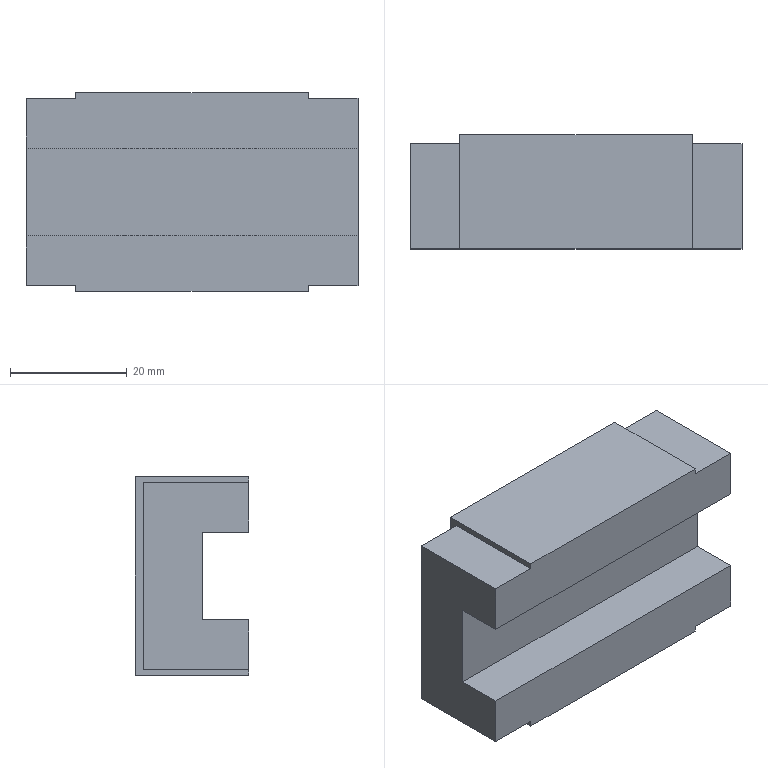Part | NX | 1 solid | 30 faces | box 56.8 x 19.5 x 34 mm | volume 29007 mm3 | plane 18 | cone 8 | cylinder 4 | commonest cylinder face diameters 3.3 x4
STEP:
#1=CARTESIAN_POINT('',(8.5,8.25,-16.));
#2=VERTEX_POINT('',#1);
#3=CARTESIAN_POINT('',(8.5,-9.75,-16.));
#4=VERTEX_POINT('',#3);
#5=CARTESIAN_POINT('',(8.5,8.25,-16.));
#6=DIRECTION('',(0.,-1.,0.));
#7=VECTOR('',#6,1.);
#8=LINE('',#5,#7);
#9=EDGE_CURVE('',#2,#4,#8,.T.);
#10=ORIENTED_EDGE('',*,*,#9,.T.);
#11=CARTESIAN_POINT('',(0.,-9.75,-16.));
#12=VERTEX_POINT('',#11);
#13=CARTESIAN_POINT('',(56.8,-9.75,-16.));
#14=DIRECTION('',(-1.,0.,0.));
#15=VECTOR('',#14,1.);
#16=LINE('',#13,#15);
#17=EDGE_CURVE('',#4,#12,#16,.T.);
#18=ORIENTED_EDGE('',*,*,#17,.T.);
#19=CARTESIAN_POINT('',(0.,8.25,-16.));
#20=VERTEX_POINT('',#19);
#21=CARTESIAN_POINT('',(0.,-9.75,-16.));
#22=DIRECTION('',(0.,1.,0.));
#23=VECTOR('',#22,1.);
#24=LINE('',#21,#23);
#25=EDGE_CURVE('',#12,#20,#24,.T.);
#26=ORIENTED_EDGE('',*,*,#25,.T.);
#27=CARTESIAN_POINT('',(56.8,8.25,-16.));
#28=DIRECTION('',(-1.,0.,0.));
#29=VECTOR('',#28,1.);
#30=LINE('',#27,#29);
#31=EDGE_CURVE('',#2,#20,#30,.T.);
#32=ORIENTED_EDGE('',*,*,#31,.F.);
#33=EDGE_LOOP('',(#10,#18,#26,#32));
#34=FACE_OUTER_BOUND('',#33,.T.);
#35=CARTESIAN_POINT('',(56.8,-9.75,-16.));
#36=DIRECTION('',(0.,0.,1.));
#37=DIRECTION('',(-1.,0.,0.));
#38=AXIS2_PLACEMENT_3D('',#35,#36,#37);
#39=PLANE('',#38);
#40=ADVANCED_FACE('',(#34),#39,.F.);
#41=CARTESIAN_POINT('',(8.5,8.25,16.));
#42=VERTEX_POINT('',#41);
#43=CARTESIAN_POINT('',(8.5,8.25,16.));
#44=DIRECTION('',(0.,0.,-1.));
#45=VECTOR('',#44,1.);
#46=LINE('',#43,#45);
#47=EDGE_CURVE('',#42,#2,#46,.T.);
#48=ORIENTED_EDGE('',*,*,#47,.T.);
#49=ORIENTED_EDGE('',*,*,#31,.T.);
#50=CARTESIAN_POINT('',(0.,8.25,16.));
#51=VERTEX_POINT('',#50);
#52=CARTESIAN_POINT('',(0.,8.25,-16.));
#53=DIRECTION('',(0.,0.,1.));
#54=VECTOR('',#53,1.);
#55=LINE('',#52,#54);
#56=EDGE_CURVE('',#20,#51,#55,.T.);
#57=ORIENTED_EDGE('',*,*,#56,.T.);
#58=CARTESIAN_POINT('',(56.8,8.25,16.));
#59=DIRECTION('',(-1.,0.,0.));
#60=VECTOR('',#59,1.);
#61=LINE('',#58,#60);
#62=EDGE_CURVE('',#42,#51,#61,.T.);
#63=ORIENTED_EDGE('',*,*,#62,.F.);
#64=EDGE_LOOP('',(#48,#49,#57,#63));
#65=FACE_OUTER_BOUND('',#64,.T.);
#66=CARTESIAN_POINT('',(56.8,8.25,-16.));
#67=DIRECTION('',(0.,-1.,0.));
#68=DIRECTION('',(0.,0.,1.));
#69=AXIS2_PLACEMENT_3D('',#66,#67,#68);
#70=PLANE('',#69);
#71=ADVANCED_FACE('',(#65),#70,.F.);
#72=CARTESIAN_POINT('',(8.5,-9.75,16.));
#73=VERTEX_POINT('',#72);
#74=CARTESIAN_POINT('',(8.5,-9.75,16.));
#75=DIRECTION('',(0.,1.,0.));
#76=VECTOR('',#75,1.);
#77=LINE('',#74,#76);
#78=EDGE_CURVE('',#73,#42,#77,.T.);
#79=ORIENTED_EDGE('',*,*,#78,.T.);
#80=ORIENTED_EDGE('',*,*,#62,.T.);
#81=CARTESIAN_POINT('',(0.,-9.75,16.));
#82=VERTEX_POINT('',#81);
#83=CARTESIAN_POINT('',(0.,8.25,16.));
#84=DIRECTION('',(0.,-1.,0.));
#85=VECTOR('',#84,1.);
#86=LINE('',#83,#85);
#87=EDGE_CURVE('',#51,#82,#86,.T.);
#88=ORIENTED_EDGE('',*,*,#87,.T.);
#89=CARTESIAN_POINT('',(56.8,-9.75,16.));
#90=DIRECTION('',(-1.,0.,0.));
#91=VECTOR('',#90,1.);
#92=LINE('',#89,#91);
#93=EDGE_CURVE('',#73,#82,#92,.T.);
#94=ORIENTED_EDGE('',*,*,#93,.F.);
#95=EDGE_LOOP('',(#79,#80,#88,#94));
#96=FACE_OUTER_BOUND('',#95,.T.);
#97=CARTESIAN_POINT('',(56.8,8.25,16.));
#98=DIRECTION('',(0.,0.,-1.));
#99=DIRECTION('',(1.,0.,0.));
#100=AXIS2_PLACEMENT_3D('',#97,#98,#99);
#101=PLANE('',#100);
#102=ADVANCED_FACE('',(#96),#101,.F.);
#103=CARTESIAN_POINT('',(0.,-9.75,-7.5));
#104=VERTEX_POINT('',#103);
#105=CARTESIAN_POINT('',(0.,-9.75,-7.5));
#106=DIRECTION('',(0.,0.,-1.));
#107=VECTOR('',#106,1.);
#108=LINE('',#105,#107);
#109=EDGE_CURVE('',#104,#12,#108,.T.);
#110=ORIENTED_EDGE('',*,*,#109,.T.);
#111=ORIENTED_EDGE('',*,*,#17,.F.);
#112=CARTESIAN_POINT('',(8.5,-9.75,-17.));
#113=VERTEX_POINT('',#112);
#114=CARTESIAN_POINT('',(8.5,-9.75,-16.));
#115=DIRECTION('',(0.,0.,-1.));
#116=VECTOR('',#115,1.);
#117=LINE('',#114,#116);
#118=EDGE_CURVE('',#4,#113,#117,.T.);
#119=ORIENTED_EDGE('',*,*,#118,.T.);
#120=CARTESIAN_POINT('',(48.3,-9.75,-17.));
#121=VERTEX_POINT('',#120);
#122=CARTESIAN_POINT('',(48.3,-9.75,-17.));
#123=DIRECTION('',(-1.,0.,0.));
#124=VECTOR('',#123,1.);
#125=LINE('',#122,#124);
#126=EDGE_CURVE('',#121,#113,#125,.T.);
#127=ORIENTED_EDGE('',*,*,#126,.F.);
#128=CARTESIAN_POINT('',(48.3,-9.75,-16.));
#129=VERTEX_POINT('',#128);
#130=CARTESIAN_POINT('',(48.3,-9.75,-16.));
#131=DIRECTION('',(0.,0.,-1.));
#132=VECTOR('',#131,1.);
#133=LINE('',#130,#132);
#134=EDGE_CURVE('',#129,#121,#133,.T.);
#135=ORIENTED_EDGE('',*,*,#134,.F.);
#136=CARTESIAN_POINT('',(56.8,-9.75,-16.));
#137=VERTEX_POINT('',#136);
#138=CARTESIAN_POINT('',(56.8,-9.75,-16.));
#139=DIRECTION('',(-1.,0.,0.));
#140=VECTOR('',#139,1.);
#141=LINE('',#138,#140);
#142=EDGE_CURVE('',#137,#129,#141,.T.);
#143=ORIENTED_EDGE('',*,*,#142,.F.);
#144=CARTESIAN_POINT('',(56.8,-9.75,-7.5));
#145=VERTEX_POINT('',#144);
#146=CARTESIAN_POINT('',(56.8,-9.75,-7.5));
#147=DIRECTION('',(0.,0.,-1.));
#148=VECTOR('',#147,1.);
#149=LINE('',#146,#148);
#150=EDGE_CURVE('',#145,#137,#149,.T.);
#151=ORIENTED_EDGE('',*,*,#150,.F.);
#152=CARTESIAN_POINT('',(56.8,-9.75,-7.5));
#153=DIRECTION('',(-1.,0.,0.));
#154=VECTOR('',#153,1.);
#155=LINE('',#152,#154);
#156=EDGE_CURVE('',#145,#104,#155,.T.);
#157=ORIENTED_EDGE('',*,*,#156,.T.);
#158=EDGE_LOOP('',(#110,#111,#119,#127,#135,#143,#151,#157));
#159=FACE_OUTER_BOUND('',#158,.T.);
#160=CARTESIAN_POINT('',(56.8,-9.75,-7.5));
#161=DIRECTION('',(0.,1.,0.));
#162=DIRECTION('',(0.,0.,-1.));
#163=AXIS2_PLACEMENT_3D('',#160,#161,#162);
#164=PLANE('',#163);
#165=ADVANCED_FACE('',(#159),#164,.F.);
#166=ORIENTED_EDGE('',*,*,#142,.T.);
#167=CARTESIAN_POINT('',(48.3,8.25,-16.));
#168=VERTEX_POINT('',#167);
#169=CARTESIAN_POINT('',(48.3,8.25,-16.));
#170=DIRECTION('',(0.,-1.,0.));
#171=VECTOR('',#170,1.);
#172=LINE('',#169,#171);
#173=EDGE_CURVE('',#168,#129,#172,.T.);
#174=ORIENTED_EDGE('',*,*,#173,.F.);
#175=CARTESIAN_POINT('',(56.8,8.25,-16.));
#176=VERTEX_POINT('',#175);
#177=CARTESIAN_POINT('',(56.8,8.25,-16.));
#178=DIRECTION('',(-1.,0.,0.));
#179=VECTOR('',#178,1.);
#180=LINE('',#177,#179);
#181=EDGE_CURVE('',#176,#168,#180,.T.);
#182=ORIENTED_EDGE('',*,*,#181,.F.);
#183=CARTESIAN_POINT('',(56.8,-9.75,-16.));
#184=DIRECTION('',(0.,1.,0.));
#185=VECTOR('',#184,1.);
#186=LINE('',#183,#185);
#187=EDGE_CURVE('',#137,#176,#186,.T.);
#188=ORIENTED_EDGE('',*,*,#187,.F.);
#189=EDGE_LOOP('',(#166,#174,#182,#188));
#190=FACE_OUTER_BOUND('',#189,.T.);
#191=CARTESIAN_POINT('',(56.8,-9.75,-16.));
#192=DIRECTION('',(0.,0.,1.));
#193=DIRECTION('',(-1.,0.,0.));
#194=AXIS2_PLACEMENT_3D('',#191,#192,#193);
#195=PLANE('',#194);
#196=ADVANCED_FACE('',(#190),#195,.F.);
#197=ORIENTED_EDGE('',*,*,#181,.T.);
#198=CARTESIAN_POINT('',(48.3,8.25,16.));
#199=VERTEX_POINT('',#198);
#200=CARTESIAN_POINT('',(48.3,8.25,16.));
#201=DIRECTION('',(0.,0.,-1.));
#202=VECTOR('',#201,1.);
#203=LINE('',#200,#202);
#204=EDGE_CURVE('',#199,#168,#203,.T.);
#205=ORIENTED_EDGE('',*,*,#204,.F.);
#206=CARTESIAN_POINT('',(56.8,8.25,16.));
#207=VERTEX_POINT('',#206);
#208=CARTESIAN_POINT('',(56.8,8.25,16.));
#209=DIRECTION('',(-1.,0.,0.));
#210=VECTOR('',#209,1.);
#211=LINE('',#208,#210);
#212=EDGE_CURVE('',#207,#199,#211,.T.);
#213=ORIENTED_EDGE('',*,*,#212,.F.);
#214=CARTESIAN_POINT('',(56.8,8.25,-16.));
#215=DIRECTION('',(0.,0.,1.));
#216=VECTOR('',#215,1.);
#217=LINE('',#214,#216);
#218=EDGE_CURVE('',#176,#207,#217,.T.);
#219=ORIENTED_EDGE('',*,*,#218,.F.);
#220=EDGE_LOOP('',(#197,#205,#213,#219));
#221=FACE_OUTER_BOUND('',#220,.T.);
#222=CARTESIAN_POINT('',(56.8,8.25,-16.));
#223=DIRECTION('',(0.,-1.,0.));
#224=DIRECTION('',(0.,0.,1.));
#225=AXIS2_PLACEMENT_3D('',#222,#223,#224);
#226=PLANE('',#225);
#227=ADVANCED_FACE('',(#221),#226,.F.);
#228=ORIENTED_EDGE('',*,*,#212,.T.);
#229=CARTESIAN_POINT('',(48.3,-9.75,16.));
#230=VERTEX_POINT('',#229);
#231=CARTESIAN_POINT('',(48.3,-9.75,16.));
#232=DIRECTION('',(0.,1.,0.));
#233=VECTOR('',#232,1.);
#234=LINE('',#231,#233);
#235=EDGE_CURVE('',#230,#199,#234,.T.);
#236=ORIENTED_EDGE('',*,*,#235,.F.);
#237=CARTESIAN_POINT('',(56.8,-9.75,16.));
#238=VERTEX_POINT('',#237);
#239=CARTESIAN_POINT('',(56.8,-9.75,16.));
#240=DIRECTION('',(-1.,0.,0.));
#241=VECTOR('',#240,1.);
#242=LINE('',#239,#241);
#243=EDGE_CURVE('',#238,#230,#242,.T.);
#244=ORIENTED_EDGE('',*,*,#243,.F.);
#245=CARTESIAN_POINT('',(56.8,8.25,16.));
#246=DIRECTION('',(0.,-1.,0.));
#247=VECTOR('',#246,1.);
#248=LINE('',#245,#247);
#249=EDGE_CURVE('',#207,#238,#248,.T.);
#250=ORIENTED_EDGE('',*,*,#249,.F.);
#251=EDGE_LOOP('',(#228,#236,#244,#250));
#252=FACE_OUTER_BOUND('',#251,.T.);
#253=CARTESIAN_POINT('',(56.8,8.25,16.));
#254=DIRECTION('',(0.,0.,-1.));
#255=DIRECTION('',(1.,0.,0.));
#256=AXIS2_PLACEMENT_3D('',#253,#254,#255);
#257=PLANE('',#256);
#258=ADVANCED_FACE('',(#252),#257,.F.);
#259=CARTESIAN_POINT('',(0.,-9.75,7.5));
#260=VERTEX_POINT('',#259);
#261=CARTESIAN_POINT('',(0.,-9.75,16.));
#262=DIRECTION('',(0.,0.,-1.));
#263=VECTOR('',#262,1.);
#264=LINE('',#261,#263);
#265=EDGE_CURVE('',#82,#260,#264,.T.);
#266=ORIENTED_EDGE('',*,*,#265,.T.);
#267=CARTESIAN_POINT('',(56.8,-9.75,7.5));
#268=VERTEX_POINT('',#267);
#269=CARTESIAN_POINT('',(56.8,-9.75,7.5));
#270=DIRECTION('',(-1.,0.,0.));
#271=VECTOR('',#270,1.);
#272=LINE('',#269,#271);
#273=EDGE_CURVE('',#268,#260,#272,.T.);
#274=ORIENTED_EDGE('',*,*,#273,.F.);
#275=CARTESIAN_POINT('',(56.8,-9.75,16.));
#276=DIRECTION('',(0.,0.,-1.));
#277=VECTOR('',#276,1.);
#278=LINE('',#275,#277);
#279=EDGE_CURVE('',#238,#268,#278,.T.);
#280=ORIENTED_EDGE('',*,*,#279,.F.);
#281=ORIENTED_EDGE('',*,*,#243,.T.);
#282=CARTESIAN_POINT('',(48.3,-9.75,17.));
#283=VERTEX_POINT('',#282);
#284=CARTESIAN_POINT('',(48.3,-9.75,17.));
#285=DIRECTION('',(0.,0.,-1.));
#286=VECTOR('',#285,1.);
#287=LINE('',#284,#286);
#288=EDGE_CURVE('',#283,#230,#287,.T.);
#289=ORIENTED_EDGE('',*,*,#288,.F.);
#290=CARTESIAN_POINT('',(8.5,-9.75,17.));
#291=VERTEX_POINT('',#290);
#292=CARTESIAN_POINT('',(48.3,-9.75,17.));
#293=DIRECTION('',(-1.,0.,0.));
#294=VECTOR('',#293,1.);
#295=LINE('',#292,#294);
#296=EDGE_CURVE('',#283,#291,#295,.T.);
#297=ORIENTED_EDGE('',*,*,#296,.T.);
#298=CARTESIAN_POINT('',(8.5,-9.75,17.));
#299=DIRECTION('',(0.,0.,-1.));
#300=VECTOR('',#299,1.);
#301=LINE('',#298,#300);
#302=EDGE_CURVE('',#291,#73,#301,.T.);
#303=ORIENTED_EDGE('',*,*,#302,.T.);
#304=ORIENTED_EDGE('',*,*,#93,.T.);
#305=EDGE_LOOP('',(#266,#274,#280,#281,#289,#297,#303,#304));
#306=FACE_OUTER_BOUND('',#305,.T.);
#307=CARTESIAN_POINT('',(56.8,-9.75,16.));
#308=DIRECTION('',(0.,1.,0.));
#309=DIRECTION('',(0.,0.,-1.));
#310=AXIS2_PLACEMENT_3D('',#307,#308,#309);
#311=PLANE('',#310);
#312=ADVANCED_FACE('',(#306),#311,.F.);
#313=CARTESIAN_POINT('',(0.,-1.75,7.5));
#314=VERTEX_POINT('',#313);
#315=CARTESIAN_POINT('',(0.,-9.75,7.5));
#316=DIRECTION('',(0.,1.,0.));
#317=VECTOR('',#316,1.);
#318=LINE('',#315,#317);
#319=EDGE_CURVE('',#260,#314,#318,.T.);
#320=ORIENTED_EDGE('',*,*,#319,.T.);
#321=CARTESIAN_POINT('',(56.8,-1.75,7.5));
#322=VERTEX_POINT('',#321);
#323=CARTESIAN_POINT('',(56.8,-1.75,7.5));
#324=DIRECTION('',(-1.,0.,0.));
#325=VECTOR('',#324,1.);
#326=LINE('',#323,#325);
#327=EDGE_CURVE('',#322,#314,#326,.T.);
#328=ORIENTED_EDGE('',*,*,#327,.F.);
#329=CARTESIAN_POINT('',(56.8,-9.75,7.5));
#330=DIRECTION('',(0.,1.,0.));
#331=VECTOR('',#330,1.);
#332=LINE('',#329,#331);
#333=EDGE_CURVE('',#268,#322,#332,.T.);
#334=ORIENTED_EDGE('',*,*,#333,.F.);
#335=ORIENTED_EDGE('',*,*,#273,.T.);
#336=EDGE_LOOP('',(#320,#328,#334,#335));
#337=FACE_OUTER_BOUND('',#336,.T.);
#338=CARTESIAN_POINT('',(56.8,-9.75,7.5));
#339=DIRECTION('',(0.,0.,1.));
#340=DIRECTION('',(0.,1.,0.));
#341=AXIS2_PLACEMENT_3D('',#338,#339,#340);
#342=PLANE('',#341);
#343=ADVANCED_FACE('',(#337),#342,.F.);
#344=CARTESIAN_POINT('',(0.,-1.75,-7.5));
#345=VERTEX_POINT('',#344);
#346=CARTESIAN_POINT('',(0.,-1.75,7.5));
#347=DIRECTION('',(0.,0.,-1.));
#348=VECTOR('',#347,1.);
#349=LINE('',#346,#348);
#350=EDGE_CURVE('',#314,#345,#349,.T.);
#351=ORIENTED_EDGE('',*,*,#350,.T.);
#352=CARTESIAN_POINT('',(56.8,-1.75,-7.5));
#353=VERTEX_POINT('',#352);
#354=CARTESIAN_POINT('',(56.8,-1.75,-7.5));
#355=DIRECTION('',(-1.,0.,0.));
#356=VECTOR('',#355,1.);
#357=LINE('',#354,#356);
#358=EDGE_CURVE('',#353,#345,#357,.T.);
#359=ORIENTED_EDGE('',*,*,#358,.F.);
#360=CARTESIAN_POINT('',(56.8,-1.75,7.5));
#361=DIRECTION('',(0.,0.,-1.));
#362=VECTOR('',#361,1.);
#363=LINE('',#360,#362);
#364=EDGE_CURVE('',#322,#353,#363,.T.);
#365=ORIENTED_EDGE('',*,*,#364,.F.);
#366=ORIENTED_EDGE('',*,*,#327,.T.);
#367=EDGE_LOOP('',(#351,#359,#365,#366));
#368=FACE_OUTER_BOUND('',#367,.T.);
#369=CARTESIAN_POINT('',(56.8,-1.75,7.5));
#370=DIRECTION('',(0.,1.,0.));
#371=DIRECTION('',(0.,0.,-1.));
#372=AXIS2_PLACEMENT_3D('',#369,#370,#371);
#373=PLANE('',#372);
#374=ADVANCED_FACE('',(#368),#373,.F.);
#375=CARTESIAN_POINT('',(0.,-1.75,-7.5));
#376=DIRECTION('',(0.,-1.,0.));
#377=VECTOR('',#376,1.);
#378=LINE('',#375,#377);
#379=EDGE_CURVE('',#345,#104,#378,.T.);
#380=ORIENTED_EDGE('',*,*,#379,.T.);
#381=ORIENTED_EDGE('',*,*,#156,.F.);
#382=CARTESIAN_POINT('',(56.8,-1.75,-7.5));
#383=DIRECTION('',(0.,-1.,0.));
#384=VECTOR('',#383,1.);
#385=LINE('',#382,#384);
#386=EDGE_CURVE('',#353,#145,#385,.T.);
#387=ORIENTED_EDGE('',*,*,#386,.F.);
#388=ORIENTED_EDGE('',*,*,#358,.T.);
#389=EDGE_LOOP('',(#380,#381,#387,#388));
#390=FACE_OUTER_BOUND('',#389,.T.);
#391=CARTESIAN_POINT('',(56.8,-1.75,-7.5));
#392=DIRECTION('',(0.,0.,-1.));
#393=DIRECTION('',(0.,-1.,0.));
#394=AXIS2_PLACEMENT_3D('',#391,#392,#393);
#395=PLANE('',#394);
#396=ADVANCED_FACE('',(#390),#395,.F.);
#397=ORIENTED_EDGE('',*,*,#150,.T.);
#398=ORIENTED_EDGE('',*,*,#187,.T.);
#399=ORIENTED_EDGE('',*,*,#218,.T.);
#400=ORIENTED_EDGE('',*,*,#249,.T.);
#401=ORIENTED_EDGE('',*,*,#279,.T.);
#402=ORIENTED_EDGE('',*,*,#333,.T.);
#403=ORIENTED_EDGE('',*,*,#364,.T.);
#404=ORIENTED_EDGE('',*,*,#386,.T.);
#405=EDGE_LOOP('',(#397,#398,#399,#400,#401,#402,#403,#404));
#406=FACE_OUTER_BOUND('',#405,.T.);
#407=CARTESIAN_POINT('',(56.8,0.,0.));
#408=DIRECTION('',(1.,0.,0.));
#409=DIRECTION('',(0.,0.,1.));
#410=AXIS2_PLACEMENT_3D('',#407,#408,#409);
#411=PLANE('',#410);
#412=ADVANCED_FACE('',(#406),#411,.T.);
#413=ORIENTED_EDGE('',*,*,#109,.F.);
#414=ORIENTED_EDGE('',*,*,#379,.F.);
#415=ORIENTED_EDGE('',*,*,#350,.F.);
#416=ORIENTED_EDGE('',*,*,#319,.F.);
#417=ORIENTED_EDGE('',*,*,#265,.F.);
#418=ORIENTED_EDGE('',*,*,#87,.F.);
#419=ORIENTED_EDGE('',*,*,#56,.F.);
#420=ORIENTED_EDGE('',*,*,#25,.F.);
#421=EDGE_LOOP('',(#413,#414,#415,#416,#417,#418,#419,#420));
#422=FACE_OUTER_BOUND('',#421,.T.);
#423=CARTESIAN_POINT('',(0.,0.,0.));
#424=DIRECTION('',(1.,0.,0.));
#425=DIRECTION('',(0.,0.,1.));
#426=AXIS2_PLACEMENT_3D('',#423,#424,#425);
#427=PLANE('',#426);
#428=ADVANCED_FACE('',(#422),#427,.F.);
#429=CARTESIAN_POINT('',(8.5,9.75,-17.));
#430=VERTEX_POINT('',#429);
#431=CARTESIAN_POINT('',(8.5,-9.75,-17.));
#432=DIRECTION('',(0.,1.,0.));
#433=VECTOR('',#432,1.);
#434=LINE('',#431,#433);
#435=EDGE_CURVE('',#113,#430,#434,.T.);
#436=ORIENTED_EDGE('',*,*,#435,.T.);
#437=CARTESIAN_POINT('',(48.3,9.75,-17.));
#438=VERTEX_POINT('',#437);
#439=CARTESIAN_POINT('',(48.3,9.75,-17.));
#440=DIRECTION('',(-1.,0.,0.));
#441=VECTOR('',#440,1.);
#442=LINE('',#439,#441);
#443=EDGE_CURVE('',#438,#430,#442,.T.);
#444=ORIENTED_EDGE('',*,*,#443,.F.);
#445=CARTESIAN_POINT('',(48.3,-9.75,-17.));
#446=DIRECTION('',(0.,1.,0.));
#447=VECTOR('',#446,1.);
#448=LINE('',#445,#447);
#449=EDGE_CURVE('',#121,#438,#448,.T.);
#450=ORIENTED_EDGE('',*,*,#449,.F.);
#451=ORIENTED_EDGE('',*,*,#126,.T.);
#452=EDGE_LOOP('',(#436,#444,#450,#451));
#453=FACE_OUTER_BOUND('',#452,.T.);
#454=CARTESIAN_POINT('',(48.3,-9.75,-17.));
#455=DIRECTION('',(0.,0.,1.));
#456=DIRECTION('',(-1.,0.,0.));
#457=AXIS2_PLACEMENT_3D('',#454,#455,#456);
#458=PLANE('',#457);
#459=ADVANCED_FACE('',(#453),#458,.F.);
#460=CARTESIAN_POINT('',(41.4,9.75,11.));
#461=VERTEX_POINT('',#460);
#462=CARTESIAN_POINT('',(41.4,9.75,13.));
#463=DIRECTION('',(0.,-1.,0.));
#464=DIRECTION('',(0.,0.,-1.));
#465=AXIS2_PLACEMENT_3D('',#462,#463,#464);
#466=CIRCLE('',#465,2.);
#467=EDGE_CURVE('',#461,#461,#466,.T.);
#468=ORIENTED_EDGE('',*,*,#467,.T.);
#469=EDGE_LOOP('',(#468));
#470=FACE_BOUND('',#469,.T.);
#471=CARTESIAN_POINT('',(41.4,9.75,-15.));
#472=VERTEX_POINT('',#471);
#473=CARTESIAN_POINT('',(41.4,9.75,-13.));
#474=DIRECTION('',(0.,-1.,0.));
#475=DIRECTION('',(0.,0.,-1.));
#476=AXIS2_PLACEMENT_3D('',#473,#474,#475);
#477=CIRCLE('',#476,2.);
#478=EDGE_CURVE('',#472,#472,#477,.T.);
#479=ORIENTED_EDGE('',*,*,#478,.T.);
#480=EDGE_LOOP('',(#479));
#481=FACE_BOUND('',#480,.T.);
#482=CARTESIAN_POINT('',(15.4,9.75,11.));
#483=VERTEX_POINT('',#482);
#484=CARTESIAN_POINT('',(15.4,9.75,13.));
#485=DIRECTION('',(0.,-1.,0.));
#486=DIRECTION('',(0.,0.,-1.));
#487=AXIS2_PLACEMENT_3D('',#484,#485,#486);
#488=CIRCLE('',#487,2.);
#489=EDGE_CURVE('',#483,#483,#488,.T.);
#490=ORIENTED_EDGE('',*,*,#489,.T.);
#491=EDGE_LOOP('',(#490));
#492=FACE_BOUND('',#491,.T.);
#493=CARTESIAN_POINT('',(15.4,9.75,-15.));
#494=VERTEX_POINT('',#493);
#495=CARTESIAN_POINT('',(15.4,9.75,-13.));
#496=DIRECTION('',(0.,-1.,0.));
#497=DIRECTION('',(0.,0.,-1.));
#498=AXIS2_PLACEMENT_3D('',#495,#496,#497);
#499=CIRCLE('',#498,2.);
#500=EDGE_CURVE('',#494,#494,#499,.T.);
#501=ORIENTED_EDGE('',*,*,#500,.T.);
#502=EDGE_LOOP('',(#501));
#503=FACE_BOUND('',#502,.T.);
#504=CARTESIAN_POINT('',(8.5,9.75,17.));
#505=VERTEX_POINT('',#504);
#506=CARTESIAN_POINT('',(8.5,9.75,-17.));
#507=DIRECTION('',(0.,0.,1.));
#508=VECTOR('',#507,1.);
#509=LINE('',#506,#508);
#510=EDGE_CURVE('',#430,#505,#509,.T.);
#511=ORIENTED_EDGE('',*,*,#510,.T.);
#512=CARTESIAN_POINT('',(48.3,9.75,17.));
#513=VERTEX_POINT('',#512);
#514=CARTESIAN_POINT('',(48.3,9.75,17.));
#515=DIRECTION('',(-1.,0.,0.));
#516=VECTOR('',#515,1.);
#517=LINE('',#514,#516);
#518=EDGE_CURVE('',#513,#505,#517,.T.);
#519=ORIENTED_EDGE('',*,*,#518,.F.);
#520=CARTESIAN_POINT('',(48.3,9.75,-17.));
#521=DIRECTION('',(0.,0.,1.));
#522=VECTOR('',#521,1.);
#523=LINE('',#520,#522);
#524=EDGE_CURVE('',#438,#513,#523,.T.);
#525=ORIENTED_EDGE('',*,*,#524,.F.);
#526=ORIENTED_EDGE('',*,*,#443,.T.);
#527=EDGE_LOOP('',(#511,#519,#525,#526));
#528=FACE_BOUND('',#527,.T.);
#529=CARTESIAN_POINT('',(48.3,9.75,-17.));
#530=DIRECTION('',(0.,-1.,0.));
#531=DIRECTION('',(0.,0.,1.));
#532=AXIS2_PLACEMENT_3D('',#529,#530,#531);
#533=PLANE('',#532);
#534=ADVANCED_FACE('',(#470,#481,#492,#503,#528),#533,.F.);
#535=CARTESIAN_POINT('',(8.5,9.75,17.));
#536=DIRECTION('',(0.,-1.,0.));
#537=VECTOR('',#536,1.);
#538=LINE('',#535,#537);
#539=EDGE_CURVE('',#505,#291,#538,.T.);
#540=ORIENTED_EDGE('',*,*,#539,.T.);
#541=ORIENTED_EDGE('',*,*,#296,.F.);
#542=CARTESIAN_POINT('',(48.3,9.75,17.));
#543=DIRECTION('',(0.,-1.,0.));
#544=VECTOR('',#543,1.);
#545=LINE('',#542,#544);
#546=EDGE_CURVE('',#513,#283,#545,.T.);
#547=ORIENTED_EDGE('',*,*,#546,.F.);
#548=ORIENTED_EDGE('',*,*,#518,.T.);
#549=EDGE_LOOP('',(#540,#541,#547,#548));
#550=FACE_OUTER_BOUND('',#549,.T.);
#551=CARTESIAN_POINT('',(48.3,9.75,17.));
#552=DIRECTION('',(0.,0.,-1.));
#553=DIRECTION('',(1.,0.,0.));
#554=AXIS2_PLACEMENT_3D('',#551,#552,#553);
#555=PLANE('',#554);
#556=ADVANCED_FACE('',(#550),#555,.F.);
#557=ORIENTED_EDGE('',*,*,#134,.T.);
#558=ORIENTED_EDGE('',*,*,#449,.T.);
#559=ORIENTED_EDGE('',*,*,#524,.T.);
#560=ORIENTED_EDGE('',*,*,#546,.T.);
#561=ORIENTED_EDGE('',*,*,#288,.T.);
#562=ORIENTED_EDGE('',*,*,#235,.T.);
#563=ORIENTED_EDGE('',*,*,#204,.T.);
#564=ORIENTED_EDGE('',*,*,#173,.T.);
#565=EDGE_LOOP('',(#557,#558,#559,#560,#561,#562,#563,#564));
#566=FACE_OUTER_BOUND('',#565,.T.);
#567=CARTESIAN_POINT('',(48.3,0.,0.));
#568=DIRECTION('',(1.,0.,0.));
#569=DIRECTION('',(0.,0.,1.));
#570=AXIS2_PLACEMENT_3D('',#567,#568,#569);
#571=PLANE('',#570);
#572=ADVANCED_FACE('',(#566),#571,.T.);
#573=ORIENTED_EDGE('',*,*,#118,.F.);
#574=ORIENTED_EDGE('',*,*,#9,.F.);
#575=ORIENTED_EDGE('',*,*,#47,.F.);
#576=ORIENTED_EDGE('',*,*,#78,.F.);
#577=ORIENTED_EDGE('',*,*,#302,.F.);
#578=ORIENTED_EDGE('',*,*,#539,.F.);
#579=ORIENTED_EDGE('',*,*,#510,.F.);
#580=ORIENTED_EDGE('',*,*,#435,.F.);
#581=EDGE_LOOP('',(#573,#574,#575,#576,#577,#578,#579,#580));
#582=FACE_OUTER_BOUND('',#581,.T.);
#583=CARTESIAN_POINT('',(8.5,0.,0.));
#584=DIRECTION('',(1.,0.,0.));
#585=DIRECTION('',(0.,0.,1.));
#586=AXIS2_PLACEMENT_3D('',#583,#584,#585);
#587=PLANE('',#586);
#588=ADVANCED_FACE('',(#582),#587,.F.);
#589=CARTESIAN_POINT('',(15.4,-0.25,-14.65));
#590=VERTEX_POINT('',#589);
#591=CARTESIAN_POINT('',(15.4,-0.25,-13.));
#592=DIRECTION('',(0.,1.,0.));
#593=DIRECTION('',(0.,0.,-1.));
#594=AXIS2_PLACEMENT_3D('',#591,#592,#593);
#595=CIRCLE('',#594,1.65);
#596=EDGE_CURVE('',#590,#590,#595,.T.);
#597=ORIENTED_EDGE('',*,*,#596,.T.);
#598=EDGE_LOOP('',(#597));
#599=FACE_BOUND('',#598,.T.);
#600=CARTESIAN_POINT('',(15.4,-1.241,-13.));
#601=VERTEX_POINT('',#600);
#602=VERTEX_LOOP('',#601);
#603=FACE_BOUND('',#602,.T.);
#604=CARTESIAN_POINT('',(15.4,-0.25,-13.));
#605=DIRECTION('',(0.,1.,0.));
#606=DIRECTION('',(0.,0.,-1.));
#607=AXIS2_PLACEMENT_3D('',#604,#605,#606);
#608=CONICAL_SURFACE('',#607,1.65,59.);
#609=ADVANCED_FACE('',(#599,#603),#608,.F.);
#610=CARTESIAN_POINT('',(15.4,9.4,-14.65));
#611=VERTEX_POINT('',#610);
#612=CARTESIAN_POINT('',(15.4,9.4,-13.));
#613=DIRECTION('',(0.,1.,0.));
#614=DIRECTION('',(0.,0.,-1.));
#615=AXIS2_PLACEMENT_3D('',#612,#613,#614);
#616=CIRCLE('',#615,1.65);
#617=EDGE_CURVE('',#611,#611,#616,.T.);
#618=ORIENTED_EDGE('',*,*,#617,.T.);
#619=EDGE_LOOP('',(#618));
#620=FACE_BOUND('',#619,.T.);
#621=ORIENTED_EDGE('',*,*,#596,.F.);
#622=EDGE_LOOP('',(#621));
#623=FACE_BOUND('',#622,.T.);
#624=CARTESIAN_POINT('',(15.4,9.75,-13.));
#625=DIRECTION('',(0.,-1.,0.));
#626=DIRECTION('',(0.,0.,1.));
#627=AXIS2_PLACEMENT_3D('',#624,#625,#626);
#628=CYLINDRICAL_SURFACE('',#627,1.65);
#629=ADVANCED_FACE('',(#620,#623),#628,.F.);
#630=ORIENTED_EDGE('',*,*,#617,.F.);
#631=EDGE_LOOP('',(#630));
#632=FACE_BOUND('',#631,.T.);
#633=ORIENTED_EDGE('',*,*,#500,.F.);
#634=EDGE_LOOP('',(#633));
#635=FACE_BOUND('',#634,.T.);
#636=CARTESIAN_POINT('',(15.4,9.75,-13.));
#637=DIRECTION('',(0.,1.,0.));
#638=DIRECTION('',(0.,0.,-1.));
#639=AXIS2_PLACEMENT_3D('',#636,#637,#638);
#640=CONICAL_SURFACE('',#639,2.,45.);
#641=ADVANCED_FACE('',(#632,#635),#640,.F.);
#642=CARTESIAN_POINT('',(15.4,-0.25,11.35));
#643=VERTEX_POINT('',#642);
#644=CARTESIAN_POINT('',(15.4,-0.25,13.));
#645=DIRECTION('',(0.,1.,0.));
#646=DIRECTION('',(0.,0.,-1.));
#647=AXIS2_PLACEMENT_3D('',#644,#645,#646);
#648=CIRCLE('',#647,1.65);
#649=EDGE_CURVE('',#643,#643,#648,.T.);
#650=ORIENTED_EDGE('',*,*,#649,.T.);
#651=EDGE_LOOP('',(#650));
#652=FACE_BOUND('',#651,.T.);
#653=CARTESIAN_POINT('',(15.4,-1.241,13.));
#654=VERTEX_POINT('',#653);
#655=VERTEX_LOOP('',#654);
#656=FACE_BOUND('',#655,.T.);
#657=CARTESIAN_POINT('',(15.4,-0.25,13.));
#658=DIRECTION('',(0.,1.,0.));
#659=DIRECTION('',(0.,0.,-1.));
#660=AXIS2_PLACEMENT_3D('',#657,#658,#659);
#661=CONICAL_SURFACE('',#660,1.65,59.);
#662=ADVANCED_FACE('',(#652,#656),#661,.F.);
#663=CARTESIAN_POINT('',(15.4,9.4,11.35));
#664=VERTEX_POINT('',#663);
#665=CARTESIAN_POINT('',(15.4,9.4,13.));
#666=DIRECTION('',(0.,1.,0.));
#667=DIRECTION('',(0.,0.,-1.));
#668=AXIS2_PLACEMENT_3D('',#665,#666,#667);
#669=CIRCLE('',#668,1.65);
#670=EDGE_CURVE('',#664,#664,#669,.T.);
#671=ORIENTED_EDGE('',*,*,#670,.T.);
#672=EDGE_LOOP('',(#671));
#673=FACE_BOUND('',#672,.T.);
#674=ORIENTED_EDGE('',*,*,#649,.F.);
#675=EDGE_LOOP('',(#674));
#676=FACE_BOUND('',#675,.T.);
#677=CARTESIAN_POINT('',(15.4,9.75,13.));
#678=DIRECTION('',(0.,-1.,0.));
#679=DIRECTION('',(0.,0.,1.));
#680=AXIS2_PLACEMENT_3D('',#677,#678,#679);
#681=CYLINDRICAL_SURFACE('',#680,1.65);
#682=ADVANCED_FACE('',(#673,#676),#681,.F.);
#683=ORIENTED_EDGE('',*,*,#670,.F.);
#684=EDGE_LOOP('',(#683));
#685=FACE_BOUND('',#684,.T.);
#686=ORIENTED_EDGE('',*,*,#489,.F.);
#687=EDGE_LOOP('',(#686));
#688=FACE_BOUND('',#687,.T.);
#689=CARTESIAN_POINT('',(15.4,9.75,13.));
#690=DIRECTION('',(0.,1.,0.));
#691=DIRECTION('',(0.,0.,-1.));
#692=AXIS2_PLACEMENT_3D('',#689,#690,#691);
#693=CONICAL_SURFACE('',#692,2.,45.);
#694=ADVANCED_FACE('',(#685,#688),#693,.F.);
#695=CARTESIAN_POINT('',(41.4,-0.25,-14.65));
#696=VERTEX_POINT('',#695);
#697=CARTESIAN_POINT('',(41.4,-0.25,-13.));
#698=DIRECTION('',(0.,1.,0.));
#699=DIRECTION('',(0.,0.,-1.));
#700=AXIS2_PLACEMENT_3D('',#697,#698,#699);
#701=CIRCLE('',#700,1.65);
#702=EDGE_CURVE('',#696,#696,#701,.T.);
#703=ORIENTED_EDGE('',*,*,#702,.T.);
#704=EDGE_LOOP('',(#703));
#705=FACE_BOUND('',#704,.T.);
#706=CARTESIAN_POINT('',(41.4,-1.241,-13.));
#707=VERTEX_POINT('',#706);
#708=VERTEX_LOOP('',#707);
#709=FACE_BOUND('',#708,.T.);
#710=CARTESIAN_POINT('',(41.4,-0.25,-13.));
#711=DIRECTION('',(0.,1.,0.));
#712=DIRECTION('',(0.,0.,-1.));
#713=AXIS2_PLACEMENT_3D('',#710,#711,#712);
#714=CONICAL_SURFACE('',#713,1.65,59.);
#715=ADVANCED_FACE('',(#705,#709),#714,.F.);
#716=CARTESIAN_POINT('',(41.4,9.4,-14.65));
#717=VERTEX_POINT('',#716);
#718=CARTESIAN_POINT('',(41.4,9.4,-13.));
#719=DIRECTION('',(0.,1.,0.));
#720=DIRECTION('',(0.,0.,-1.));
#721=AXIS2_PLACEMENT_3D('',#718,#719,#720);
#722=CIRCLE('',#721,1.65);
#723=EDGE_CURVE('',#717,#717,#722,.T.);
#724=ORIENTED_EDGE('',*,*,#723,.T.);
#725=EDGE_LOOP('',(#724));
#726=FACE_BOUND('',#725,.T.);
#727=ORIENTED_EDGE('',*,*,#702,.F.);
#728=EDGE_LOOP('',(#727));
#729=FACE_BOUND('',#728,.T.);
#730=CARTESIAN_POINT('',(41.4,9.75,-13.));
#731=DIRECTION('',(0.,-1.,0.));
#732=DIRECTION('',(0.,0.,1.));
#733=AXIS2_PLACEMENT_3D('',#730,#731,#732);
#734=CYLINDRICAL_SURFACE('',#733,1.65);
#735=ADVANCED_FACE('',(#726,#729),#734,.F.);
#736=ORIENTED_EDGE('',*,*,#723,.F.);
#737=EDGE_LOOP('',(#736));
#738=FACE_BOUND('',#737,.T.);
#739=ORIENTED_EDGE('',*,*,#478,.F.);
#740=EDGE_LOOP('',(#739));
#741=FACE_BOUND('',#740,.T.);
#742=CARTESIAN_POINT('',(41.4,9.75,-13.));
#743=DIRECTION('',(0.,1.,0.));
#744=DIRECTION('',(0.,0.,-1.));
#745=AXIS2_PLACEMENT_3D('',#742,#743,#744);
#746=CONICAL_SURFACE('',#745,2.,45.);
#747=ADVANCED_FACE('',(#738,#741),#746,.F.);
#748=CARTESIAN_POINT('',(41.4,-0.25,11.35));
#749=VERTEX_POINT('',#748);
#750=CARTESIAN_POINT('',(41.4,-0.25,13.));
#751=DIRECTION('',(0.,1.,0.));
#752=DIRECTION('',(0.,0.,-1.));
#753=AXIS2_PLACEMENT_3D('',#750,#751,#752);
#754=CIRCLE('',#753,1.65);
#755=EDGE_CURVE('',#749,#749,#754,.T.);
#756=ORIENTED_EDGE('',*,*,#755,.T.);
#757=EDGE_LOOP('',(#756));
#758=FACE_BOUND('',#757,.T.);
#759=CARTESIAN_POINT('',(41.4,-1.241,13.));
#760=VERTEX_POINT('',#759);
#761=VERTEX_LOOP('',#760);
#762=FACE_BOUND('',#761,.T.);
#763=CARTESIAN_POINT('',(41.4,-0.25,13.));
#764=DIRECTION('',(0.,1.,0.));
#765=DIRECTION('',(0.,0.,-1.));
#766=AXIS2_PLACEMENT_3D('',#763,#764,#765);
#767=CONICAL_SURFACE('',#766,1.65,59.);
#768=ADVANCED_FACE('',(#758,#762),#767,.F.);
#769=CARTESIAN_POINT('',(41.4,9.4,11.35));
#770=VERTEX_POINT('',#769);
#771=CARTESIAN_POINT('',(41.4,9.4,13.));
#772=DIRECTION('',(0.,1.,0.));
#773=DIRECTION('',(0.,0.,-1.));
#774=AXIS2_PLACEMENT_3D('',#771,#772,#773);
#775=CIRCLE('',#774,1.65);
#776=EDGE_CURVE('',#770,#770,#775,.T.);
#777=ORIENTED_EDGE('',*,*,#776,.T.);
#778=EDGE_LOOP('',(#777));
#779=FACE_BOUND('',#778,.T.);
#780=ORIENTED_EDGE('',*,*,#755,.F.);
#781=EDGE_LOOP('',(#780));
#782=FACE_BOUND('',#781,.T.);
#783=CARTESIAN_POINT('',(41.4,9.75,13.));
#784=DIRECTION('',(0.,-1.,0.));
#785=DIRECTION('',(0.,0.,1.));
#786=AXIS2_PLACEMENT_3D('',#783,#784,#785);
#787=CYLINDRICAL_SURFACE('',#786,1.65);
#788=ADVANCED_FACE('',(#779,#782),#787,.F.);
#789=ORIENTED_EDGE('',*,*,#776,.F.);
#790=EDGE_LOOP('',(#789));
#791=FACE_BOUND('',#790,.T.);
#792=ORIENTED_EDGE('',*,*,#467,.F.);
#793=EDGE_LOOP('',(#792));
#794=FACE_BOUND('',#793,.T.);
#795=CARTESIAN_POINT('',(41.4,9.75,13.));
#796=DIRECTION('',(0.,1.,0.));
#797=DIRECTION('',(0.,0.,-1.));
#798=AXIS2_PLACEMENT_3D('',#795,#796,#797);
#799=CONICAL_SURFACE('',#798,2.,45.);
#800=ADVANCED_FACE('',(#791,#794),#799,.F.);
#801=CLOSED_SHELL('',(#40,#71,#102,#165,#196,#227,#258,#312,#343,#374,#396,#412,#428,#459,#534,#556,#572,#588,#609,#629,#641,#662,#682,#694,#715,#735,#747,#768,#788,#800));
#802=MANIFOLD_SOLID_BREP('',#801);
#803=(LENGTH_UNIT()NAMED_UNIT(*)SI_UNIT(.MILLI.,.METRE.));
#804=UNCERTAINTY_MEASURE_WITH_UNIT(LENGTH_MEASURE(0.00002),#803,'','');
#805=(NAMED_UNIT(*)PLANE_ANGLE_UNIT()SI_UNIT($,.RADIAN.));
#806=PLANE_ANGLE_MEASURE_WITH_UNIT(PLANE_ANGLE_MEASURE(0.01745),#805);
#807=DIMENSIONAL_EXPONENTS(0.,0.,0.,0.,0.,0.,0.);
#808=(CONVERSION_BASED_UNIT('DEGREE',#806)NAMED_UNIT(#807)PLANE_ANGLE_UNIT());
#809=(NAMED_UNIT(*)SI_UNIT($,.STERADIAN.)SOLID_ANGLE_UNIT());
#810=(GEOMETRIC_REPRESENTATION_CONTEXT(3)GLOBAL_UNCERTAINTY_ASSIGNED_CONTEXT((#804))GLOBAL_UNIT_ASSIGNED_CONTEXT((#803,#808,#809))REPRESENTATION_CONTEXT('',''));
#811=ADVANCED_BREP_SHAPE_REPRESENTATION('',(#802),#810);